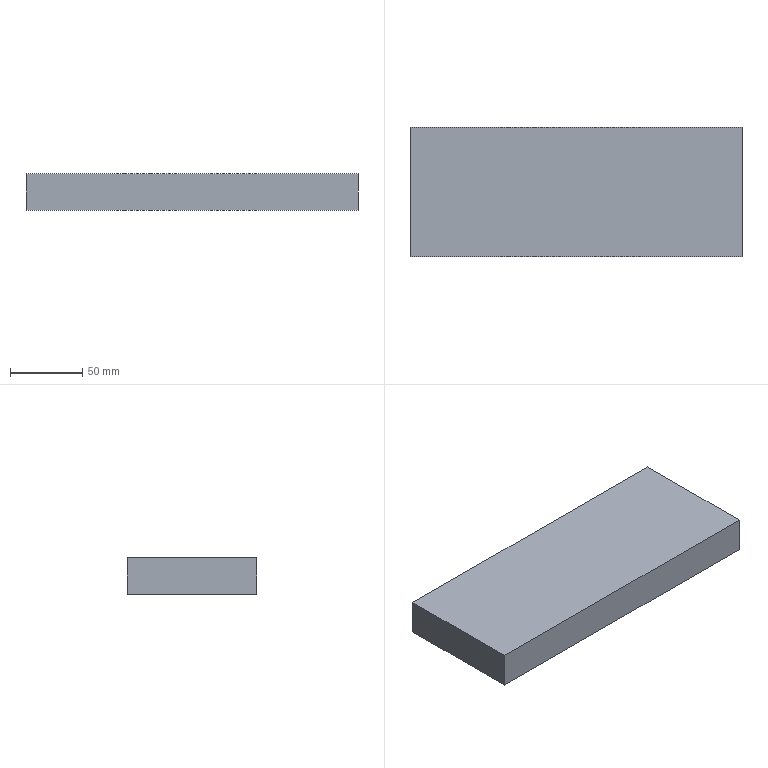Part | SolidWorks | features Extrusion 1 | 1 solid | 6 faces | box 230 x 90 x 25 mm | volume 517500 mm3 | plane 6
STEP:
#1=CARTESIAN_POINT('',(0.,0.,0.));
#2=VERTEX_POINT('',#1);
#3=CARTESIAN_POINT('',(0.,90.,0.));
#4=VERTEX_POINT('',#3);
#5=CARTESIAN_POINT('',(0.,0.,0.));
#6=DIRECTION('',(0.,1.,0.));
#7=VECTOR('',#6,1000.);
#8=LINE('',#5,#7);
#9=EDGE_CURVE('',#2,#4,#8,.T.);
#10=ORIENTED_EDGE('',*,*,#9,.T.);
#11=CARTESIAN_POINT('',(0.,90.,25.));
#12=VERTEX_POINT('',#11);
#13=CARTESIAN_POINT('',(0.,90.,25.));
#14=DIRECTION('',(0.,0.,-1.));
#15=VECTOR('',#14,1000.);
#16=LINE('',#13,#15);
#17=EDGE_CURVE('',#12,#4,#16,.T.);
#18=ORIENTED_EDGE('',*,*,#17,.F.);
#19=CARTESIAN_POINT('',(0.,0.,25.));
#20=VERTEX_POINT('',#19);
#21=CARTESIAN_POINT('',(0.,0.,25.));
#22=DIRECTION('',(0.,1.,0.));
#23=VECTOR('',#22,1000.);
#24=LINE('',#21,#23);
#25=EDGE_CURVE('',#20,#12,#24,.T.);
#26=ORIENTED_EDGE('',*,*,#25,.F.);
#27=CARTESIAN_POINT('',(0.,0.,25.));
#28=DIRECTION('',(0.,0.,-1.));
#29=VECTOR('',#28,1000.);
#30=LINE('',#27,#29);
#31=EDGE_CURVE('',#20,#2,#30,.T.);
#32=ORIENTED_EDGE('',*,*,#31,.T.);
#33=EDGE_LOOP('',(#10,#18,#26,#32));
#34=FACE_OUTER_BOUND('',#33,.T.);
#35=CARTESIAN_POINT('',(0.,0.,25.));
#36=DIRECTION('',(-1.,0.,0.));
#37=DIRECTION('',(0.,0.,1.));
#38=AXIS2_PLACEMENT_3D('',#35,#36,#37);
#39=PLANE('',#38);
#40=ADVANCED_FACE('',(#34),#39,.F.);
#41=CARTESIAN_POINT('',(-230.,90.,0.));
#42=VERTEX_POINT('',#41);
#43=CARTESIAN_POINT('',(0.,90.,0.));
#44=DIRECTION('',(-1.,0.,0.));
#45=VECTOR('',#44,1000.);
#46=LINE('',#43,#45);
#47=EDGE_CURVE('',#4,#42,#46,.T.);
#48=ORIENTED_EDGE('',*,*,#47,.T.);
#49=CARTESIAN_POINT('',(-230.,90.,25.));
#50=VERTEX_POINT('',#49);
#51=CARTESIAN_POINT('',(-230.,90.,25.));
#52=DIRECTION('',(0.,0.,-1.));
#53=VECTOR('',#52,1000.);
#54=LINE('',#51,#53);
#55=EDGE_CURVE('',#50,#42,#54,.T.);
#56=ORIENTED_EDGE('',*,*,#55,.F.);
#57=CARTESIAN_POINT('',(0.,90.,25.));
#58=DIRECTION('',(-1.,0.,0.));
#59=VECTOR('',#58,1000.);
#60=LINE('',#57,#59);
#61=EDGE_CURVE('',#12,#50,#60,.T.);
#62=ORIENTED_EDGE('',*,*,#61,.F.);
#63=ORIENTED_EDGE('',*,*,#17,.T.);
#64=EDGE_LOOP('',(#48,#56,#62,#63));
#65=FACE_OUTER_BOUND('',#64,.T.);
#66=CARTESIAN_POINT('',(0.,90.,25.));
#67=DIRECTION('',(0.,-1.,0.));
#68=DIRECTION('',(1.,0.,0.));
#69=AXIS2_PLACEMENT_3D('',#66,#67,#68);
#70=PLANE('',#69);
#71=ADVANCED_FACE('',(#65),#70,.F.);
#72=CARTESIAN_POINT('',(-230.,0.,0.));
#73=VERTEX_POINT('',#72);
#74=CARTESIAN_POINT('',(-230.,0.,0.));
#75=DIRECTION('',(0.,-1.,0.));
#76=VECTOR('',#75,1000.);
#77=LINE('',#74,#76);
#78=EDGE_CURVE('',#42,#73,#77,.T.);
#79=ORIENTED_EDGE('',*,*,#78,.T.);
#80=CARTESIAN_POINT('',(-230.,0.,25.));
#81=VERTEX_POINT('',#80);
#82=CARTESIAN_POINT('',(-230.,0.,25.));
#83=DIRECTION('',(0.,0.,-1.));
#84=VECTOR('',#83,1000.);
#85=LINE('',#82,#84);
#86=EDGE_CURVE('',#81,#73,#85,.T.);
#87=ORIENTED_EDGE('',*,*,#86,.F.);
#88=CARTESIAN_POINT('',(-230.,0.,25.));
#89=DIRECTION('',(0.,-1.,0.));
#90=VECTOR('',#89,1000.);
#91=LINE('',#88,#90);
#92=EDGE_CURVE('',#50,#81,#91,.T.);
#93=ORIENTED_EDGE('',*,*,#92,.F.);
#94=ORIENTED_EDGE('',*,*,#55,.T.);
#95=EDGE_LOOP('',(#79,#87,#93,#94));
#96=FACE_OUTER_BOUND('',#95,.T.);
#97=CARTESIAN_POINT('',(-230.,0.,25.));
#98=DIRECTION('',(1.,0.,0.));
#99=DIRECTION('',(0.,0.,-1.));
#100=AXIS2_PLACEMENT_3D('',#97,#98,#99);
#101=PLANE('',#100);
#102=ADVANCED_FACE('',(#96),#101,.F.);
#103=CARTESIAN_POINT('',(0.,0.,0.));
#104=DIRECTION('',(1.,0.,0.));
#105=VECTOR('',#104,1000.);
#106=LINE('',#103,#105);
#107=EDGE_CURVE('',#73,#2,#106,.T.);
#108=ORIENTED_EDGE('',*,*,#107,.T.);
#109=ORIENTED_EDGE('',*,*,#31,.F.);
#110=CARTESIAN_POINT('',(0.,0.,25.));
#111=DIRECTION('',(1.,0.,0.));
#112=VECTOR('',#111,1000.);
#113=LINE('',#110,#112);
#114=EDGE_CURVE('',#81,#20,#113,.T.);
#115=ORIENTED_EDGE('',*,*,#114,.F.);
#116=ORIENTED_EDGE('',*,*,#86,.T.);
#117=EDGE_LOOP('',(#108,#109,#115,#116));
#118=FACE_OUTER_BOUND('',#117,.T.);
#119=CARTESIAN_POINT('',(0.,0.,25.));
#120=DIRECTION('',(0.,1.,0.));
#121=DIRECTION('',(0.,0.,1.));
#122=AXIS2_PLACEMENT_3D('',#119,#120,#121);
#123=PLANE('',#122);
#124=ADVANCED_FACE('',(#118),#123,.F.);
#125=ORIENTED_EDGE('',*,*,#25,.T.);
#126=ORIENTED_EDGE('',*,*,#61,.T.);
#127=ORIENTED_EDGE('',*,*,#92,.T.);
#128=ORIENTED_EDGE('',*,*,#114,.T.);
#129=EDGE_LOOP('',(#125,#126,#127,#128));
#130=FACE_OUTER_BOUND('',#129,.T.);
#131=CARTESIAN_POINT('',(0.,0.,25.));
#132=DIRECTION('',(0.,0.,1.));
#133=DIRECTION('',(1.,0.,0.));
#134=AXIS2_PLACEMENT_3D('',#131,#132,#133);
#135=PLANE('',#134);
#136=ADVANCED_FACE('',(#130),#135,.T.);
#137=ORIENTED_EDGE('',*,*,#9,.F.);
#138=ORIENTED_EDGE('',*,*,#107,.F.);
#139=ORIENTED_EDGE('',*,*,#78,.F.);
#140=ORIENTED_EDGE('',*,*,#47,.F.);
#141=EDGE_LOOP('',(#137,#138,#139,#140));
#142=FACE_OUTER_BOUND('',#141,.T.);
#143=CARTESIAN_POINT('',(0.,0.,0.));
#144=DIRECTION('',(0.,0.,1.));
#145=DIRECTION('',(1.,0.,0.));
#146=AXIS2_PLACEMENT_3D('',#143,#144,#145);
#147=PLANE('',#146);
#148=ADVANCED_FACE('',(#142),#147,.F.);
#149=CLOSED_SHELL('',(#40,#71,#102,#124,#136,#148));
#150=MANIFOLD_SOLID_BREP('',#149);
#151=CARTESIAN_POINT('',(0.,0.,0.));
#152=DIRECTION('',(0.,0.,1.));
#153=DIRECTION('',(1.,0.,0.));
#154=AXIS2_PLACEMENT_3D('',#151,#152,#153);
#155=(LENGTH_UNIT()NAMED_UNIT(*)SI_UNIT(.MILLI.,.METRE.));
#156=UNCERTAINTY_MEASURE_WITH_UNIT(LENGTH_MEASURE(0.00001),#155,'','');
#157=(NAMED_UNIT(*)PLANE_ANGLE_UNIT()SI_UNIT($,.RADIAN.));
#158=(NAMED_UNIT(*)SI_UNIT($,.STERADIAN.)SOLID_ANGLE_UNIT());
#159=(GEOMETRIC_REPRESENTATION_CONTEXT(3)GLOBAL_UNCERTAINTY_ASSIGNED_CONTEXT((#156))GLOBAL_UNIT_ASSIGNED_CONTEXT((#155,#157,#158))REPRESENTATION_CONTEXT('',''));
#160=ADVANCED_BREP_SHAPE_REPRESENTATION('',(#150,#154),#159);